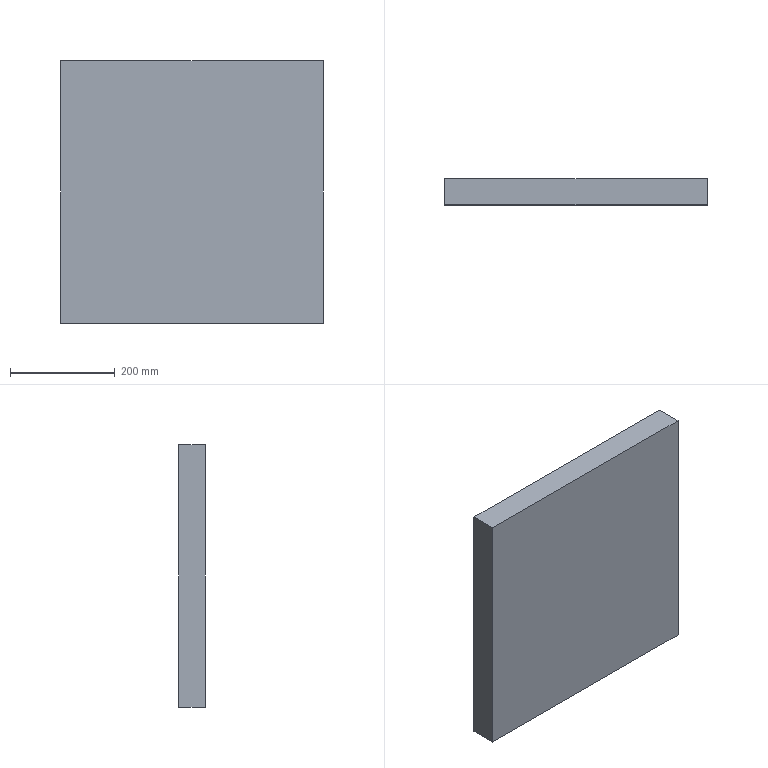Part | SolidWorks | features Extrusion 1 | 1 solid | 6 faces | box 500 x 50 x 500 mm | volume 12500000 mm3 | plane 6
STEP:
#1=CARTESIAN_POINT('',(250.,0.,250.));
#2=VERTEX_POINT('',#1);
#3=CARTESIAN_POINT('',(250.,0.,-250.));
#4=VERTEX_POINT('',#3);
#5=CARTESIAN_POINT('',(250.,0.,-250.));
#6=DIRECTION('',(0.,0.,-1.));
#7=VECTOR('',#6,1000.);
#8=LINE('',#5,#7);
#9=EDGE_CURVE('',#2,#4,#8,.T.);
#10=ORIENTED_EDGE('',*,*,#9,.T.);
#11=CARTESIAN_POINT('',(250.,50.,-250.));
#12=VERTEX_POINT('',#11);
#13=CARTESIAN_POINT('',(250.,50.,-250.));
#14=DIRECTION('',(0.,-1.,0.));
#15=VECTOR('',#14,1000.);
#16=LINE('',#13,#15);
#17=EDGE_CURVE('',#12,#4,#16,.T.);
#18=ORIENTED_EDGE('',*,*,#17,.F.);
#19=CARTESIAN_POINT('',(250.,50.,250.));
#20=VERTEX_POINT('',#19);
#21=CARTESIAN_POINT('',(250.,50.,-250.));
#22=DIRECTION('',(0.,0.,-1.));
#23=VECTOR('',#22,1000.);
#24=LINE('',#21,#23);
#25=EDGE_CURVE('',#20,#12,#24,.T.);
#26=ORIENTED_EDGE('',*,*,#25,.F.);
#27=CARTESIAN_POINT('',(250.,50.,250.));
#28=DIRECTION('',(0.,-1.,0.));
#29=VECTOR('',#28,1000.);
#30=LINE('',#27,#29);
#31=EDGE_CURVE('',#20,#2,#30,.T.);
#32=ORIENTED_EDGE('',*,*,#31,.T.);
#33=EDGE_LOOP('',(#10,#18,#26,#32));
#34=FACE_OUTER_BOUND('',#33,.T.);
#35=CARTESIAN_POINT('',(250.,50.,-250.));
#36=DIRECTION('',(-1.,0.,0.));
#37=DIRECTION('',(0.,0.,1.));
#38=AXIS2_PLACEMENT_3D('',#35,#36,#37);
#39=PLANE('',#38);
#40=ADVANCED_FACE('',(#34),#39,.F.);
#41=CARTESIAN_POINT('',(-250.,0.,-250.));
#42=VERTEX_POINT('',#41);
#43=CARTESIAN_POINT('',(-250.,0.,-250.));
#44=DIRECTION('',(-1.,0.,0.));
#45=VECTOR('',#44,1000.);
#46=LINE('',#43,#45);
#47=EDGE_CURVE('',#4,#42,#46,.T.);
#48=ORIENTED_EDGE('',*,*,#47,.T.);
#49=CARTESIAN_POINT('',(-250.,50.,-250.));
#50=VERTEX_POINT('',#49);
#51=CARTESIAN_POINT('',(-250.,50.,-250.));
#52=DIRECTION('',(0.,-1.,0.));
#53=VECTOR('',#52,1000.);
#54=LINE('',#51,#53);
#55=EDGE_CURVE('',#50,#42,#54,.T.);
#56=ORIENTED_EDGE('',*,*,#55,.F.);
#57=CARTESIAN_POINT('',(-250.,50.,-250.));
#58=DIRECTION('',(-1.,0.,0.));
#59=VECTOR('',#58,1000.);
#60=LINE('',#57,#59);
#61=EDGE_CURVE('',#12,#50,#60,.T.);
#62=ORIENTED_EDGE('',*,*,#61,.F.);
#63=ORIENTED_EDGE('',*,*,#17,.T.);
#64=EDGE_LOOP('',(#48,#56,#62,#63));
#65=FACE_OUTER_BOUND('',#64,.T.);
#66=CARTESIAN_POINT('',(-250.,50.,-250.));
#67=DIRECTION('',(0.,0.,1.));
#68=DIRECTION('',(1.,0.,0.));
#69=AXIS2_PLACEMENT_3D('',#66,#67,#68);
#70=PLANE('',#69);
#71=ADVANCED_FACE('',(#65),#70,.F.);
#72=CARTESIAN_POINT('',(-250.,0.,250.));
#73=VERTEX_POINT('',#72);
#74=CARTESIAN_POINT('',(-250.,0.,-250.));
#75=DIRECTION('',(0.,0.,1.));
#76=VECTOR('',#75,1000.);
#77=LINE('',#74,#76);
#78=EDGE_CURVE('',#42,#73,#77,.T.);
#79=ORIENTED_EDGE('',*,*,#78,.T.);
#80=CARTESIAN_POINT('',(-250.,50.,250.));
#81=VERTEX_POINT('',#80);
#82=CARTESIAN_POINT('',(-250.,50.,250.));
#83=DIRECTION('',(0.,-1.,0.));
#84=VECTOR('',#83,1000.);
#85=LINE('',#82,#84);
#86=EDGE_CURVE('',#81,#73,#85,.T.);
#87=ORIENTED_EDGE('',*,*,#86,.F.);
#88=CARTESIAN_POINT('',(-250.,50.,-250.));
#89=DIRECTION('',(0.,0.,1.));
#90=VECTOR('',#89,1000.);
#91=LINE('',#88,#90);
#92=EDGE_CURVE('',#50,#81,#91,.T.);
#93=ORIENTED_EDGE('',*,*,#92,.F.);
#94=ORIENTED_EDGE('',*,*,#55,.T.);
#95=EDGE_LOOP('',(#79,#87,#93,#94));
#96=FACE_OUTER_BOUND('',#95,.T.);
#97=CARTESIAN_POINT('',(-250.,50.,-250.));
#98=DIRECTION('',(1.,0.,0.));
#99=DIRECTION('',(0.,0.,-1.));
#100=AXIS2_PLACEMENT_3D('',#97,#98,#99);
#101=PLANE('',#100);
#102=ADVANCED_FACE('',(#96),#101,.F.);
#103=CARTESIAN_POINT('',(-250.,0.,250.));
#104=DIRECTION('',(1.,0.,0.));
#105=VECTOR('',#104,1000.);
#106=LINE('',#103,#105);
#107=EDGE_CURVE('',#73,#2,#106,.T.);
#108=ORIENTED_EDGE('',*,*,#107,.T.);
#109=ORIENTED_EDGE('',*,*,#31,.F.);
#110=CARTESIAN_POINT('',(-250.,50.,250.));
#111=DIRECTION('',(1.,0.,0.));
#112=VECTOR('',#111,1000.);
#113=LINE('',#110,#112);
#114=EDGE_CURVE('',#81,#20,#113,.T.);
#115=ORIENTED_EDGE('',*,*,#114,.F.);
#116=ORIENTED_EDGE('',*,*,#86,.T.);
#117=EDGE_LOOP('',(#108,#109,#115,#116));
#118=FACE_OUTER_BOUND('',#117,.T.);
#119=CARTESIAN_POINT('',(-250.,50.,250.));
#120=DIRECTION('',(0.,0.,-1.));
#121=DIRECTION('',(-1.,0.,0.));
#122=AXIS2_PLACEMENT_3D('',#119,#120,#121);
#123=PLANE('',#122);
#124=ADVANCED_FACE('',(#118),#123,.F.);
#125=ORIENTED_EDGE('',*,*,#25,.T.);
#126=ORIENTED_EDGE('',*,*,#61,.T.);
#127=ORIENTED_EDGE('',*,*,#92,.T.);
#128=ORIENTED_EDGE('',*,*,#114,.T.);
#129=EDGE_LOOP('',(#125,#126,#127,#128));
#130=FACE_OUTER_BOUND('',#129,.T.);
#131=CARTESIAN_POINT('',(0.,50.,0.));
#132=DIRECTION('',(0.,1.,0.));
#133=DIRECTION('',(0.,0.,1.));
#134=AXIS2_PLACEMENT_3D('',#131,#132,#133);
#135=PLANE('',#134);
#136=ADVANCED_FACE('',(#130),#135,.T.);
#137=ORIENTED_EDGE('',*,*,#9,.F.);
#138=ORIENTED_EDGE('',*,*,#107,.F.);
#139=ORIENTED_EDGE('',*,*,#78,.F.);
#140=ORIENTED_EDGE('',*,*,#47,.F.);
#141=EDGE_LOOP('',(#137,#138,#139,#140));
#142=FACE_OUTER_BOUND('',#141,.T.);
#143=CARTESIAN_POINT('',(0.,0.,0.));
#144=DIRECTION('',(0.,1.,0.));
#145=DIRECTION('',(0.,0.,1.));
#146=AXIS2_PLACEMENT_3D('',#143,#144,#145);
#147=PLANE('',#146);
#148=ADVANCED_FACE('',(#142),#147,.F.);
#149=CLOSED_SHELL('',(#40,#71,#102,#124,#136,#148));
#150=MANIFOLD_SOLID_BREP('',#149);
#151=CARTESIAN_POINT('',(0.,0.,0.));
#152=DIRECTION('',(0.,0.,1.));
#153=DIRECTION('',(1.,0.,0.));
#154=AXIS2_PLACEMENT_3D('',#151,#152,#153);
#155=(LENGTH_UNIT()NAMED_UNIT(*)SI_UNIT(.MILLI.,.METRE.));
#156=UNCERTAINTY_MEASURE_WITH_UNIT(LENGTH_MEASURE(0.00001),#155,'','');
#157=(NAMED_UNIT(*)PLANE_ANGLE_UNIT()SI_UNIT($,.RADIAN.));
#158=(NAMED_UNIT(*)SI_UNIT($,.STERADIAN.)SOLID_ANGLE_UNIT());
#159=(GEOMETRIC_REPRESENTATION_CONTEXT(3)GLOBAL_UNCERTAINTY_ASSIGNED_CONTEXT((#156))GLOBAL_UNIT_ASSIGNED_CONTEXT((#155,#157,#158))REPRESENTATION_CONTEXT('',''));
#160=ADVANCED_BREP_SHAPE_REPRESENTATION('',(#150,#154),#159);